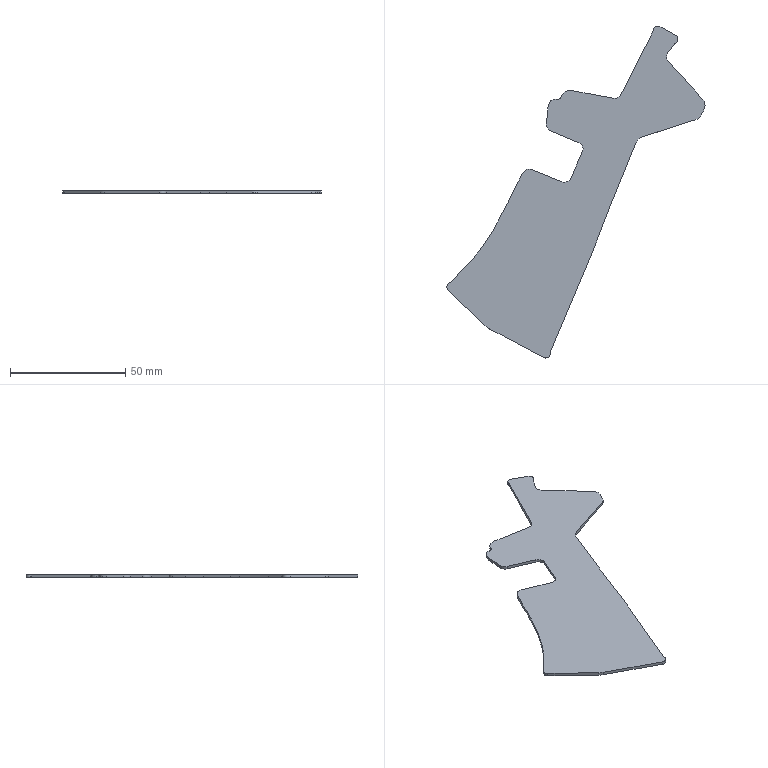Part | STEP file | gslz 2016.10.28-13_id198_x_t | 1 solid | 52 faces | box 111.925 x 143.919 x 1.25 mm | volume 6648 mm3 | plane 31 | cylinder 21 | commonest cylinder face diameters 4 x9 6 x6 8 x2 3 x1 6.078 x1 16 x1